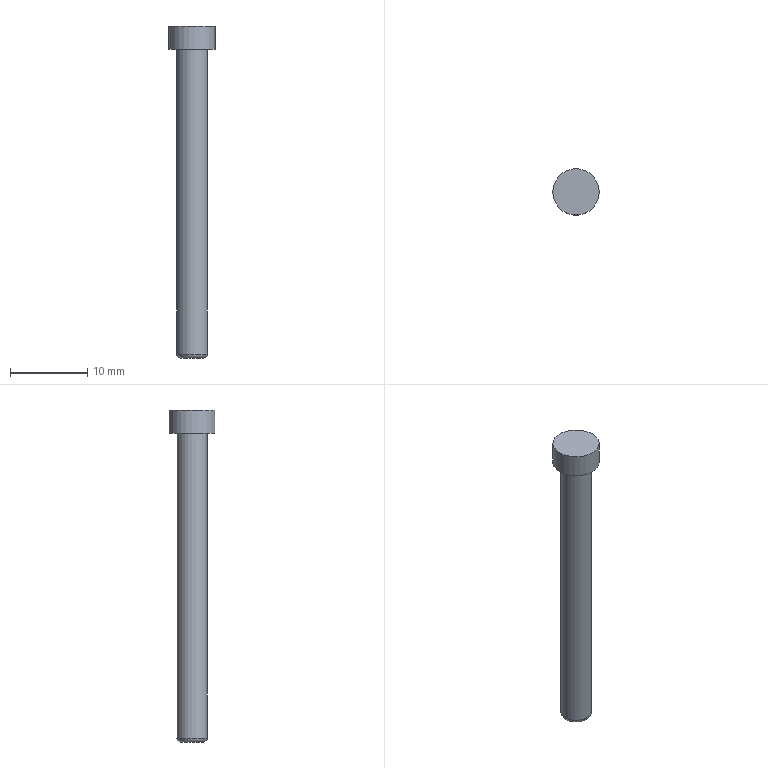Part | NX | features solid 2 | 1 solid | 6 faces | box 6 x 6 x 43 mm | volume 586.841 mm3 | plane 3 | cylinder 2 | torus 1 | commonest cylinder face diameters 4 x1 6 x1
STEP:
#1=CARTESIAN_POINT('',(63.863,31.,-10.5));
#2=VERTEX_POINT('',#1);
#3=CARTESIAN_POINT('',(65.363,31.,-10.5));
#4=DIRECTION('',(0.,0.,-1.));
#5=DIRECTION('',(-1.,0.,0.));
#6=AXIS2_PLACEMENT_3D('',#3,#4,#5);
#7=CIRCLE('',#6,1.5);
#8=EDGE_CURVE('',#2,#2,#7,.T.);
#9=ORIENTED_EDGE('',*,*,#8,.T.);
#10=EDGE_LOOP('',(#9));
#11=FACE_BOUND('',#10,.T.);
#12=CARTESIAN_POINT('',(65.363,31.,-10.5));
#13=DIRECTION('',(0.,0.,-1.));
#14=DIRECTION('',(-1.,0.,0.));
#15=AXIS2_PLACEMENT_3D('',#12,#13,#14);
#16=PLANE('',#15);
#17=ADVANCED_FACE('',(#11),#16,.T.);
#18=CARTESIAN_POINT('',(63.363,31.,29.5));
#19=VERTEX_POINT('',#18);
#20=CARTESIAN_POINT('',(65.363,31.,29.5));
#21=DIRECTION('',(0.,0.,-1.));
#22=DIRECTION('',(-1.,0.,0.));
#23=AXIS2_PLACEMENT_3D('',#20,#21,#22);
#24=CIRCLE('',#23,2.);
#25=EDGE_CURVE('',#19,#19,#24,.F.);
#26=ORIENTED_EDGE('',*,*,#25,.F.);
#27=EDGE_LOOP('',(#26));
#28=FACE_BOUND('',#27,.T.);
#29=CARTESIAN_POINT('',(63.363,31.,-10.));
#30=VERTEX_POINT('',#29);
#31=CARTESIAN_POINT('',(65.363,31.,-10.));
#32=DIRECTION('',(0.,0.,-1.));
#33=DIRECTION('',(-1.,0.,0.));
#34=AXIS2_PLACEMENT_3D('',#31,#32,#33);
#35=CIRCLE('',#34,2.);
#36=EDGE_CURVE('',#30,#30,#35,.F.);
#37=ORIENTED_EDGE('',*,*,#36,.T.);
#38=EDGE_LOOP('',(#37));
#39=FACE_BOUND('',#38,.T.);
#40=CARTESIAN_POINT('',(65.363,31.,32.5));
#41=DIRECTION('',(0.,0.,-1.));
#42=DIRECTION('',(1.,0.,0.));
#43=AXIS2_PLACEMENT_3D('',#40,#41,#42);
#44=CYLINDRICAL_SURFACE('',#43,2.);
#45=ADVANCED_FACE('',(#28,#39),#44,.T.);
#46=ORIENTED_EDGE('',*,*,#8,.F.);
#47=EDGE_LOOP('',(#46));
#48=FACE_BOUND('',#47,.T.);
#49=ORIENTED_EDGE('',*,*,#36,.F.);
#50=EDGE_LOOP('',(#49));
#51=FACE_BOUND('',#50,.T.);
#52=CARTESIAN_POINT('',(65.363,31.,-10.));
#53=DIRECTION('',(0.,0.,-1.));
#54=DIRECTION('',(-1.,0.,0.));
#55=AXIS2_PLACEMENT_3D('',#52,#53,#54);
#56=TOROIDAL_SURFACE('',#55,1.5,0.5);
#57=ADVANCED_FACE('',(#48,#51),#56,.T.);
#58=ORIENTED_EDGE('',*,*,#25,.T.);
#59=EDGE_LOOP('',(#58));
#60=FACE_BOUND('',#59,.T.);
#61=CARTESIAN_POINT('',(68.363,31.,29.5));
#62=VERTEX_POINT('',#61);
#63=CARTESIAN_POINT('',(65.363,31.,29.5));
#64=DIRECTION('',(0.,0.,1.));
#65=DIRECTION('',(1.,0.,0.));
#66=AXIS2_PLACEMENT_3D('',#63,#64,#65);
#67=CIRCLE('',#66,3.);
#68=EDGE_CURVE('',#62,#62,#67,.T.);
#69=ORIENTED_EDGE('',*,*,#68,.F.);
#70=EDGE_LOOP('',(#69));
#71=FACE_BOUND('',#70,.T.);
#72=CARTESIAN_POINT('',(65.363,31.,29.5));
#73=DIRECTION('',(0.,0.,-1.));
#74=DIRECTION('',(-1.,0.,0.));
#75=AXIS2_PLACEMENT_3D('',#72,#73,#74);
#76=PLANE('',#75);
#77=ADVANCED_FACE('',(#60,#71),#76,.T.);
#78=ORIENTED_EDGE('',*,*,#68,.T.);
#79=EDGE_LOOP('',(#78));
#80=FACE_BOUND('',#79,.T.);
#81=CARTESIAN_POINT('',(68.363,31.,32.5));
#82=VERTEX_POINT('',#81);
#83=CARTESIAN_POINT('',(65.363,31.,32.5));
#84=DIRECTION('',(0.,0.,-1.));
#85=DIRECTION('',(1.,0.,0.));
#86=AXIS2_PLACEMENT_3D('',#83,#84,#85);
#87=CIRCLE('',#86,3.);
#88=EDGE_CURVE('',#82,#82,#87,.T.);
#89=ORIENTED_EDGE('',*,*,#88,.T.);
#90=EDGE_LOOP('',(#89));
#91=FACE_BOUND('',#90,.T.);
#92=CARTESIAN_POINT('',(65.363,31.,32.5));
#93=DIRECTION('',(0.,0.,-1.));
#94=DIRECTION('',(1.,0.,0.));
#95=AXIS2_PLACEMENT_3D('',#92,#93,#94);
#96=CYLINDRICAL_SURFACE('',#95,3.);
#97=ADVANCED_FACE('',(#80,#91),#96,.T.);
#98=ORIENTED_EDGE('',*,*,#88,.F.);
#99=EDGE_LOOP('',(#98));
#100=FACE_BOUND('',#99,.T.);
#101=CARTESIAN_POINT('',(65.363,31.,32.5));
#102=DIRECTION('',(0.,0.,1.));
#103=DIRECTION('',(1.,0.,0.));
#104=AXIS2_PLACEMENT_3D('',#101,#102,#103);
#105=PLANE('',#104);
#106=ADVANCED_FACE('',(#100),#105,.T.);
#107=CLOSED_SHELL('',(#17,#45,#57,#77,#97,#106));
#108=MANIFOLD_SOLID_BREP('',#107);
#109=(LENGTH_UNIT()NAMED_UNIT(*)SI_UNIT(.MILLI.,.METRE.));
#110=UNCERTAINTY_MEASURE_WITH_UNIT(LENGTH_MEASURE(0.00001),#109,'','');
#111=(NAMED_UNIT(*)PLANE_ANGLE_UNIT()SI_UNIT($,.RADIAN.));
#112=(NAMED_UNIT(*)SI_UNIT($,.STERADIAN.)SOLID_ANGLE_UNIT());
#113=(GEOMETRIC_REPRESENTATION_CONTEXT(3)GLOBAL_UNCERTAINTY_ASSIGNED_CONTEXT((#110))GLOBAL_UNIT_ASSIGNED_CONTEXT((#109,#111,#112))REPRESENTATION_CONTEXT('',''));
#114=ADVANCED_BREP_SHAPE_REPRESENTATION('',(#108),#113);